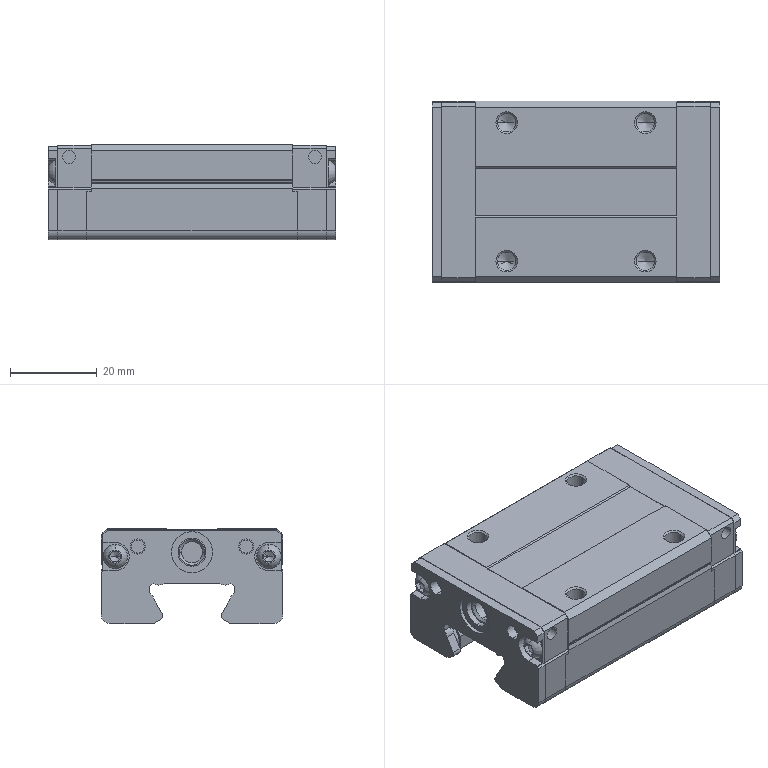Part | NX | 5 solids | 402 faces | box 66.5 x 42 x 22 mm | volume 41263 mm3 | plane 230 | cylinder 132 | cone 32 | torus 8 | commonest cylinder face diameters 3 x24 3.5 x16 6.5 x16 4 x10 1.51 x8 3.4 x8